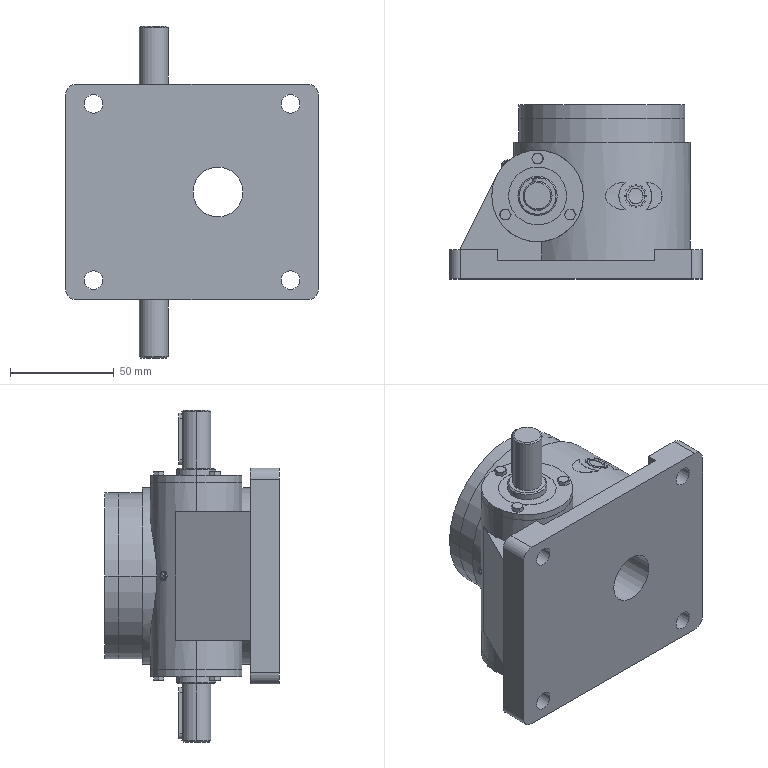Part | SolidWorks | features BaseBody 1 | 1 solid | 269 faces | box 122 x 84 x 160 mm | volume 620061 mm3 | plane 106 | cylinder 61 | cone 50 | spline 46 | torus 6 | commonest cylinder face diameters 9 x8 44.2 x7 5 x6 5.6 x4 5.88 x4 10.8 x4